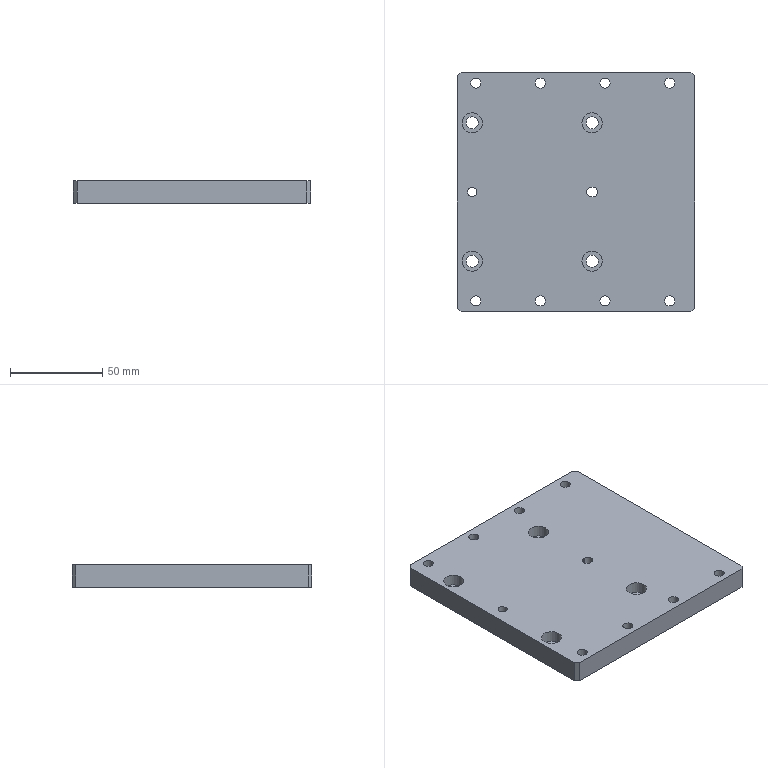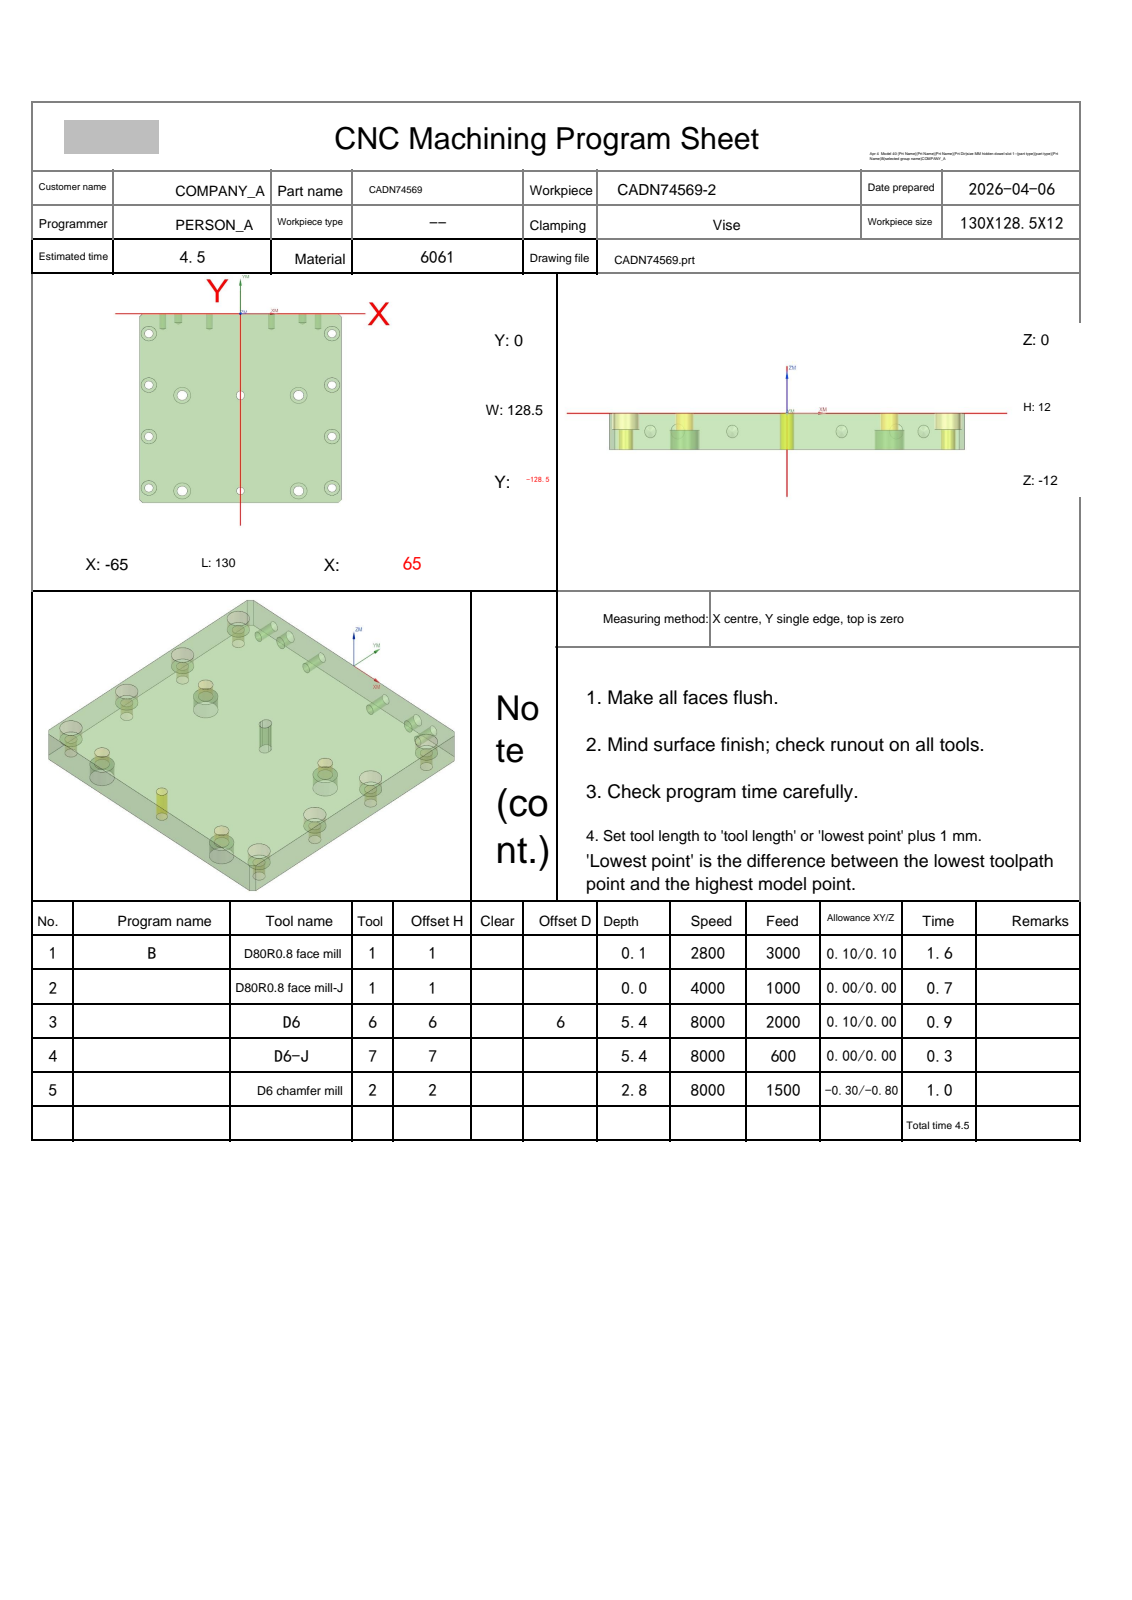NC program | NX | posted by the shop | part box 128.5 x 130 x 12 mm
Whole program:
%
O0001
(Machine time: 5.45 MIN)
(===Total Tool:4===)
(T1=D80R0.8 face mill D=80.  R=0.8  D-  H01 Z=-0.   )
(T6=D6      D=6.   R=0.   D6  H06 Z=-5.4  )
(T7=D6-J    D=6.   R=0.   D-  H07 Z=-5.4  )
(T2=D6 chamfer mill   D=6.   R=0.   D-  H02 Z=-2.8  )
G80 G90 G17 G49 G40
G91 G28 Z0
M01
N1 T01 M06
(D80R0.8 face mill  D=80. R=0.8 H=01 ce=0.10 di=0.10)
G00 G90 G54 X-117.097 Y-23.903 M03 S2800
G43 H01 Z20.
M08
Z4.517
G01 Z2.517 F3000.
X-105.097
X97.897
G02 X105.097 Y-31.103 I0.0 J-7.2
G01 Y-52.57
G02 X97.097 Y-60.57 I-8. J0.0
G01 X-97.897
G03 X-105.097 Y-67.77 I0.0 J-7.2
G01 Y-89.237
G03 X-97.097 Y-97.237 I8. J0.0
G01 X105.097
X117.097
Z4.517
G00 X-117.097 Y-23.903
Z4.033
G01 Z2.033
X-105.097
X97.897
G02 X105.097 Y-31.103 I0.0 J-7.2
G01 Y-52.57
G02 X97.097 Y-60.57 I-8. J0.0
G01 X-97.897
G03 X-105.097 Y-67.77 I0.0 J-7.2
G01 Y-89.237
G03 X-97.097 Y-97.237 I8. J0.0
G01 X105.097
X117.097
Z4.033
G00 X-117.097 Y-23.903
Z3.55
G01 Z1.55
X-105.097
X97.897
G02 X105.097 Y-31.103 I0.0 J-7.2
G01 Y-52.57
G02 X97.097 Y-60.57 I-8. J0.0
G01 X-97.897
G03 X-105.097 Y-67.77 I0.0 J-7.2
G01 Y-89.237
G03 X-97.097 Y-97.237 I8. J0.0
G01 X105.097
X117.097
Z3.55
G00 X-117.097 Y-23.903
Z3.067
G01 Z1.067
X-105.097
X97.897
G02 X105.097 Y-31.103 I0.0 J-7.2
G01 Y-52.57
G02 X97.097 Y-60.57 I-8. J0.0
G01 X-97.897
G03 X-105.097 Y-67.77 I0.0 J-7.2
G01 Y-89.237
G03 X-97.097 Y-97.237 I8. J0.0
G01 X105.097
X117.097
Z3.067
G00 Z20.
X-117.097 Y-23.903
Z2.583
G01 Z.583
X-105.097
X97.897
G02 X105.097 Y-31.103 I0.0 J-7.2
G01 Y-52.57
G02 X97.097 Y-60.57 I-8. J0.0
G01 X-97.897
G03 X-105.097 Y-67.77 I0.0 J-7.2
G01 Y-89.237
G03 X-97.097 Y-97.237 I8. J0.0
G01 X105.097
X117.097
Z2.583
G00 Z20.
X-117.097 Y-23.903
Z2.1
G01 Z.1
X-105.097
X97.897
G02 X105.097 Y-31.103 I0.0 J-7.2
G01 Y-52.57
G02 X97.097 Y-60.57 I-8. J0.0
G01 X-97.897
G03 X-105.097 Y-67.77 I0.0 J-7.2
G01 Y-89.237
G03 X-97.097 Y-97.237 I8. J0.0
G01 X105.097
X117.097
Z2.1
G00 Z20.
G91 G28 Z0.0
M05
M09
G91 G28 Z0.0
M01
N2 T01 M06
(D80R0.8 face mill-J  D=80. R=0.8 H=01 ce=0.00 di=0.00)
G00 G90 G54 X-116.999 Y-24.001 M03 S4000
G43 H01 Z20.
M08
Z2.
G01 Z0.0 F1000.
X-104.999
X97.799
G02 X104.999 Y-31.201 I0.0 J-7.2
G01 Y-52.57
G02 X96.999 Y-60.57 I-8. J0.0
G01 X-97.799
G03 X-104.999 Y-67.77 I0.0 J-7.2
G01 Y-89.139
G03 X-96.999 Y-97.139 I8. J0.0
G01 X104.999
X116.999
Z2.
G00 Z20.
G91 G28 Z0.0
M05
M09
G91 G28 Z0.0
M01
N3 T06 M06
(D6  D=6. R=0. H=06 ce=0.10 di=0.00)
G00 G90 G54 X59. Y-118.5 M03 S8000
G43 H06 Z20.
M08
Z.3
G41 D06
G01 X59.1 Y-118.507 F2000.
G03 X59.956 Y-117.556 I-.1 J.951
X59. Y-116.6 I-.956 J0.0
X59. Y-116.6 Z-.05 I0.0 J-1.9
X59. Y-116.6 Z-.4 I0.0 J-1.9
X59. Y-116.6 Z-.75 I0.0 J-1.9
X59. Y-116.6 Z-1.1 I0.0 J-1.9
X59. Y-116.6 Z-1.45 I0.0 J-1.9
X59. Y-116.6 Z-1.8 I0.0 J-1.9
X59. Y-116.6 Z-2.15 I0.0 J-1.9
X59. Y-116.6 Z-2.5 I0.0 J-1.9
X59. Y-116.6 Z-2.85 I0.0 J-1.9
X59. Y-116.6 Z-3.2 I0.0 J-1.9
X59. Y-116.6 Z-3.55 I0.0 J-1.9
X59. Y-116.6 Z-3.9 I0.0 J-1.9
X59. Y-116.6 Z-4.25 I0.0 J-1.9
X59. Y-116.6 Z-4.6 I0.0 J-1.9
X59. Y-116.6 Z-4.95 I0.0 J-1.9
X59. Y-116.6 Z-5.3 I0.0 J-1.9
X57.148 Y-118.923 Z-5.4 I0.0 J-1.9
X59. Y-120.4 I1.852 J.423
X60.9 Y-118.5 I0.0 J1.9
X59. Y-116.6 I-1.9 J0.0
X57.1 Y-118.5 I0.0 J-1.9
X57.148 Y-118.923 I1.9 J0.0
X58.08 Y-119.666 I.932 J.213
X59.036 Y-118.71 I0.0 J.956
G01 X59.029 Y-118.596
G40 X59. Y-118.5
G00 Z20.
Y-83.5
Z.3
G41 D06
G01 X59.1 Y-83.507
G03 X59.956 Y-82.556 I-.1 J.951
X59. Y-81.6 I-.956 J0.0
X59. Y-81.6 Z-.05 I0.0 J-1.9
X59. Y-81.6 Z-.4 I0.0 J-1.9
X59. Y-81.6 Z-.75 I0.0 J-1.9
X59. Y-81.6 Z-1.1 I0.0 J-1.9
X59. Y-81.6 Z-1.45 I0.0 J-1.9
X59. Y-81.6 Z-1.8 I0.0 J-1.9
X59. Y-81.6 Z-2.15 I0.0 J-1.9
X59. Y-81.6 Z-2.5 I0.0 J-1.9
X59. Y-81.6 Z-2.85 I0.0 J-1.9
X59. Y-81.6 Z-3.2 I0.0 J-1.9
X59. Y-81.6 Z-3.55 I0.0 J-1.9
X59. Y-81.6 Z-3.9 I0.0 J-1.9
X59. Y-81.6 Z-4.25 I0.0 J-1.9
X59. Y-81.6 Z-4.6 I0.0 J-1.9
X59. Y-81.6 Z-4.95 I0.0 J-1.9
X59. Y-81.6 Z-5.3 I0.0 J-1.9
X57.148 Y-83.923 Z-5.4 I0.0 J-1.9
X59. Y-85.4 I1.852 J.423
X60.9 Y-83.5 I0.0 J1.9
X59. Y-81.6 I-1.9 J0.0
X57.1 Y-83.5 I0.0 J-1.9
X57.148 Y-83.923 I1.9 J0.0
X58.08 Y-84.666 I.932 J.213
X59.036 Y-83.71 I0.0 J.956
G01 X59.029 Y-83.596
G40 X59. Y-83.5
G00 Z20.
Y-48.5
Z.3
G41 D06
G01 X59.1 Y-48.507
G03 X59.956 Y-47.556 I-.1 J.951
X59. Y-46.6 I-.956 J0.0
X59. Y-46.6 Z-.05 I0.0 J-1.9
X59. Y-46.6 Z-.4 I0.0 J-1.9
X59. Y-46.6 Z-.75 I0.0 J-1.9
X59. Y-46.6 Z-1.1 I0.0 J-1.9
X59. Y-46.6 Z-1.45 I0.0 J-1.9
X59. Y-46.6 Z-1.8 I0.0 J-1.9
X59. Y-46.6 Z-2.15 I0.0 J-1.9
X59. Y-46.6 Z-2.5 I0.0 J-1.9
X59. Y-46.6 Z-2.85 I0.0 J-1.9
X59. Y-46.6 Z-3.2 I0.0 J-1.9
X59. Y-46.6 Z-3.55 I0.0 J-1.9
X59. Y-46.6 Z-3.9 I0.0 J-1.9
X59. Y-46.6 Z-4.25 I0.0 J-1.9
X59. Y-46.6 Z-4.6 I0.0 J-1.9
X59. Y-46.6 Z-4.95 I0.0 J-1.9
X59. Y-46.6 Z-5.3 I0.0 J-1.9
X57.148 Y-48.923 Z-5.4 I0.0 J-1.9
X59. Y-50.4 I1.852 J.423
X60.9 Y-48.5 I0.0 J1.9
X59. Y-46.6 I-1.9 J0.0
X57.1 Y-48.5 I0.0 J-1.9
X57.148 Y-48.923 I1.9 J0.0
X58.08 Y-49.666 I.932 J.213
X59.036 Y-48.71 I0.0 J.956
G01 X59.029 Y-48.596
G40 X59. Y-48.5
G00 Z20.
Y-13.5
Z.3
G41 D06
G01 X59.1 Y-13.507
G03 X59.956 Y-12.556 I-.1 J.951
X59. Y-11.6 I-.956 J0.0
X59. Y-11.6 Z-.05 I0.0 J-1.9
X59. Y-11.6 Z-.4 I0.0 J-1.9
X59. Y-11.6 Z-.75 I0.0 J-1.9
X59. Y-11.6 Z-1.1 I0.0 J-1.9
X59. Y-11.6 Z-1.45 I0.0 J-1.9
X59. Y-11.6 Z-1.8 I0.0 J-1.9
X59. Y-11.6 Z-2.15 I0.0 J-1.9
X59. Y-11.6 Z-2.5 I0.0 J-1.9
X59. Y-11.6 Z-2.85 I0.0 J-1.9
X59. Y-11.6 Z-3.2 I0.0 J-1.9
X59. Y-11.6 Z-3.55 I0.0 J-1.9
X59. Y-11.6 Z-3.9 I0.0 J-1.9
X59. Y-11.6 Z-4.25 I0.0 J-1.9
X59. Y-11.6 Z-4.6 I0.0 J-1.9
X59. Y-11.6 Z-4.95 I0.0 J-1.9
X59. Y-11.6 Z-5.3 I0.0 J-1.9
X57.148 Y-13.923 Z-5.4 I0.0 J-1.9
X59. Y-15.4 I1.852 J.423
X60.9 Y-13.5 I0.0 J1.9
X59. Y-11.6 I-1.9 J0.0
X57.1 Y-13.5 I0.0 J-1.9
X57.148 Y-13.923 I1.9 J0.0
X58.08 Y-14.666 I.932 J.213
X59.036 Y-13.71 I0.0 J.956
G01 X59.029 Y-13.596
G40 X59. Y-13.5
G00 Z20.
X-59.
Z.3
G41 D06
G01 X-58.9 Y-13.507
G03 X-58.044 Y-12.556 I-.1 J.951
X-59. Y-11.6 I-.956 J0.0
X-59. Y-11.6 Z-.05 I0.0 J-1.9
X-59. Y-11.6 Z-.4 I0.0 J-1.9
X-59. Y-11.6 Z-.75 I0.0 J-1.9
X-59. Y-11.6 Z-1.1 I0.0 J-1.9
X-59. Y-11.6 Z-1.45 I0.0 J-1.9
X-59. Y-11.6 Z-1.8 I0.0 J-1.9
X-59. Y-11.6 Z-2.15 I0.0 J-1.9
X-59. Y-11.6 Z-2.5 I0.0 J-1.9
X-59. Y-11.6 Z-2.85 I0.0 J-1.9
X-59. Y-11.6 Z-3.2 I0.0 J-1.9
X-59. Y-11.6 Z-3.55 I0.0 J-1.9
X-59. Y-11.6 Z-3.9 I0.0 J-1.9
X-59. Y-11.6 Z-4.25 I0.0 J-1.9
X-59. Y-11.6 Z-4.6 I0.0 J-1.9
X-59. Y-11.6 Z-4.95 I0.0 J-1.9
X-59. Y-11.6 Z-5.3 I0.0 J-1.9
X-60.852 Y-13.923 Z-5.4 I0.0 J-1.9
X-59. Y-15.4 I1.852 J.423
X-57.1 Y-13.5 I0.0 J1.9
X-59. Y-11.6 I-1.9 J0.0
X-60.9 Y-13.5 I0.0 J-1.9
X-60.852 Y-13.923 I1.9 J0.0
X-59.92 Y-14.666 I.932 J.213
X-58.964 Y-13.71 I0.0 J.956
G01 X-58.971 Y-13.596
G40 X-59. Y-13.5
G00 Z20.
Y-48.5
Z.3
G41 D06
G01 X-58.9 Y-48.507
G03 X-58.044 Y-47.556 I-.1 J.951
X-59. Y-46.6 I-.956 J0.0
X-59. Y-46.6 Z-.05 I0.0 J-1.9
X-59. Y-46.6 Z-.4 I0.0 J-1.9
X-59. Y-46.6 Z-.75 I0.0 J-1.9
X-59. Y-46.6 Z-1.1 I0.0 J-1.9
X-59. Y-46.6 Z-1.45 I0.0 J-1.9
X-59. Y-46.6 Z-1.8 I0.0 J-1.9
X-59. Y-46.6 Z-2.15 I0.0 J-1.9
X-59. Y-46.6 Z-2.5 I0.0 J-1.9
X-59. Y-46.6 Z-2.85 I0.0 J-1.9
X-59. Y-46.6 Z-3.2 I0.0 J-1.9
X-59. Y-46.6 Z-3.55 I0.0 J-1.9
X-59. Y-46.6 Z-3.9 I0.0 J-1.9
X-59. Y-46.6 Z-4.25 I0.0 J-1.9
X-59. Y-46.6 Z-4.6 I0.0 J-1.9
X-59. Y-46.6 Z-4.95 I0.0 J-1.9
X-59. Y-46.6 Z-5.3 I0.0 J-1.9
X-60.852 Y-48.923 Z-5.4 I0.0 J-1.9
X-59. Y-50.4 I1.852 J.423
X-57.1 Y-48.5 I0.0 J1.9
X-59. Y-46.6 I-1.9 J0.0
X-60.9 Y-48.5 I0.0 J-1.9
X-60.852 Y-48.923 I1.9 J0.0
X-59.92 Y-49.666 I.932 J.213
X-58.964 Y-48.71 I0.0 J.956
G01 X-58.971 Y-48.596
G40 X-59. Y-48.5
G00 Z20.
Y-83.5
Z.3
G41 D06
G01 X-58.9 Y-83.507
G03 X-58.044 Y-82.556 I-.1 J.951
X-59. Y-81.6 I-.956 J0.0
X-59. Y-81.6 Z-.05 I0.0 J-1.9
X-59. Y-81.6 Z-.4 I0.0 J-1.9
X-59. Y-81.6 Z-.75 I0.0 J-1.9
X-59. Y-81.6 Z-1.1 I0.0 J-1.9
X-59. Y-81.6 Z-1.45 I0.0 J-1.9
X-59. Y-81.6 Z-1.8 I0.0 J-1.9
X-59. Y-81.6 Z-2.15 I0.0 J-1.9
X-59. Y-81.6 Z-2.5 I0.0 J-1.9
X-59. Y-81.6 Z-2.85 I0.0 J-1.9
X-59. Y-81.6 Z-3.2 I0.0 J-1.9
X-59. Y-81.6 Z-3.55 I0.0 J-1.9
X-59. Y-81.6 Z-3.9 I0.0 J-1.9
X-59. Y-81.6 Z-4.25 I0.0 J-1.9
X-59. Y-81.6 Z-4.6 I0.0 J-1.9
X-59. Y-81.6 Z-4.95 I0.0 J-1.9
X-59. Y-81.6 Z-5.3 I0.0 J-1.9
X-60.852 Y-83.923 Z-5.4 I0.0 J-1.9
X-59. Y-85.4 I1.852 J.423
X-57.1 Y-83.5 I0.0 J1.9
X-59. Y-81.6 I-1.9 J0.0
X-60.9 Y-83.5 I0.0 J-1.9
X-60.852 Y-83.923 I1.9 J0.0
X-59.92 Y-84.666 I.932 J.213
X-58.964 Y-83.71 I0.0 J.956
G01 X-58.971 Y-83.596
G40 X-59. Y-83.5
G00 Z20.
Y-118.5
Z.3
G41 D06
G01 X-58.9 Y-118.507
G03 X-58.044 Y-117.556 I-.1 J.951
X-59. Y-116.6 I-.956 J0.0
X-59. Y-116.6 Z-.05 I0.0 J-1.9
X-59. Y-116.6 Z-.4 I0.0 J-1.9
X-59. Y-116.6 Z-.75 I0.0 J-1.9
X-59. Y-116.6 Z-1.1 I0.0 J-1.9
X-59. Y-116.6 Z-1.45 I0.0 J-1.9
X-59. Y-116.6 Z-1.8 I0.0 J-1.9
X-59. Y-116.6 Z-2.15 I0.0 J-1.9
X-59. Y-116.6 Z-2.5 I0.0 J-1.9
X-59. Y-116.6 Z-2.85 I0.0 J-1.9
X-59. Y-116.6 Z-3.2 I0.0 J-1.9
X-59. Y-116.6 Z-3.55 I0.0 J-1.9
X-59. Y-116.6 Z-3.9 I0.0 J-1.9
X-59. Y-116.6 Z-4.25 I0.0 J-1.9
X-59. Y-116.6 Z-4.6 I0.0 J-1.9
X-59. Y-116.6 Z-4.95 I0.0 J-1.9
X-59. Y-116.6 Z-5.3 I0.0 J-1.9
X-60.852 Y-118.923 Z-5.4 I0.0 J-1.9
X-59. Y-120.4 I1.852 J.423
X-57.1 Y-118.5 I0.0 J1.9
X-59. Y-116.6 I-1.9 J0.0
X-60.9 Y-118.5 I0.0 J-1.9
X-60.852 Y-118.923 I1.9 J0.0
X-59.92 Y-119.666 I.932 J.213
X-58.964 Y-118.71 I0.0 J.956
G01 X-58.971 Y-118.596
G40 X-59. Y-118.5
G00 Z20.
G91 G28 Z0.0
M05
M09
G91 G28 Z0.0
M01
N4 T07 M06
(D6-J  D=6. R=0. H=07 ce=0.00 di=0.00)
G00 G90 G54 X59. Y-118.5 M03 S8000
G43 H07 Z20.
M08
Z-5.4
G01 X59.351 Y-116.939 F600.
X59.36 Y-116.86
G03 X59. Y-116.5 I-.36 J0.0
X57. Y-118.5 I0.0 J-2.
X59. Y-120.5 I2. J0.0
X61. Y-118.5 I0.0 J2.
X59. Y-116.5 I-2. J0.0
X58.505 Y-116.562 I0.0 J-2.
X58.234 Y-116.911 I.089 J-.349
G01 X58.274 Y-117.074
X59. Y-118.5
G00 Z20.
Y-83.5
Z-5.4
G01 X59.351 Y-81.939
X59.36 Y-81.86
G03 X59. Y-81.5 I-.36 J0.0
X57. Y-83.5 I0.0 J-2.
X59. Y-85.5 I2. J0.0
X61. Y-83.5 I0.0 J2.
X59. Y-81.5 I-2. J0.0
X58.505 Y-81.562 I0.0 J-2.
X58.234 Y-81.911 I.089 J-.349
G01 X58.274 Y-82.074
X59. Y-83.5
G00 Z20.
Y-48.5
Z-5.4
G01 X59.351 Y-46.939
X59.36 Y-46.86
G03 X59. Y-46.5 I-.36 J0.0
X57. Y-48.5 I0.0 J-2.
X59. Y-50.5 I2. J0.0
X61. Y-48.5 I0.0 J2.
X59. Y-46.5 I-2. J0.0
X58.505 Y-46.562 I0.0 J-2.
X58.234 Y-46.911 I.089 J-.349
G01 X58.274 Y-47.074
X59. Y-48.5
G00 Z20.
Y-13.5
Z-5.4
G01 X59.351 Y-11.939
X59.36 Y-11.86
G03 X59. Y-11.5 I-.36 J0.0
X57. Y-13.5 I0.0 J-2.
X59. Y-15.5 I2. J0.0
X61. Y-13.5 I0.0 J2.
X59. Y-11.5 I-2. J0.0
X58.505 Y-11.562 I0.0 J-2.
X58.234 Y-11.911 I.089 J-.349
G01 X58.274 Y-12.074
X59. Y-13.5
G00 Z20.
X-59.
Z-5.4
G01 X-58.649 Y-11.939
X-58.64 Y-11.86
G03 X-59. Y-11.5 I-.36 J0.0
X-61. Y-13.5 I0.0 J-2.
X-59. Y-15.5 I2. J0.0
X-57. Y-13.5 I0.0 J2.
X-59. Y-11.5 I-2. J0.0
X-59.495 Y-11.562 I0.0 J-2.
X-59.766 Y-11.911 I.089 J-.349
G01 X-59.726 Y-12.074
X-59. Y-13.5
G00 Z20.
Y-48.5
Z-5.4
G01 X-58.649 Y-46.939
X-58.64 Y-46.86
G03 X-59. Y-46.5 I-.36 J0.0
X-61. Y-48.5 I0.0 J-2.
X-59. Y-50.5 I2. J0.0
X-57. Y-48.5 I0.0 J2.
X-59. Y-46.5 I-2. J0.0
X-59.495 Y-46.562 I0.0 J-2.
X-59.766 Y-46.911 I.089 J-.349
G01 X-59.726 Y-47.074
X-59. Y-48.5
G00 Z20.
Y-83.5
Z-5.4
G01 X-58.649 Y-81.939
X-58.64 Y-81.86
G03 X-59. Y-81.5 I-.36 J0.0
X-61. Y-83.5 I0.0 J-2.
X-59. Y-85.5 I2. J0.0
X-57. Y-83.5 I0.0 J2.
X-59. Y-81.5 I-2. J0.0
X-59.495 Y-81.562 I0.0 J-2.
X-59.766 Y-81.911 I.089 J-.349
G01 X-59.726 Y-82.074
X-59. Y-83.5
G00 Z20.
Y-118.5
Z-5.4
G01 X-58.649 Y-116.939
X-58.64 Y-116.86
G03 X-59. Y-116.5 I-.36 J0.0
X-61. Y-118.5 I0.0 J-2.
X-59. Y-120.5 I2. J0.0
X-57. Y-118.5 I0.0 J2.
X-59. Y-116.5 I-2. J0.0
X-59.495 Y-116.562 I0.0 J-2.
X-59.766 Y-116.911 I.089 J-.349
G01 X-59.726 Y-117.074
X-59. Y-118.5
G00 Z20.
G91 G28 Z0.0
M05
M09
G91 G28 Z0.0
M01
N5 T02 M06
(D6 chamfer mill  D=6. R=0. H=02 ce=0.00 di=0.00)
G00 G90 G54 X0.0 Y-120.5 M03 S8000
G43 H02 Z20.
M08
G98 G81 X0.0 Y-120.5 Z-2.8 R3. F1000.
G80
G00 Z20.
G00 G90 X36.413 Y-56.007 M03 S8000
Z20.
Z-.9
G01 Z-1.4 F1200.
X36. Y-56.2
G03 X37.5 Y-57.7 I1.5 J0.0
X39.7 Y-55.5 I0.0 J2.2
X37.5 Y-53.3 I-2.2 J0.0
X35.3 Y-55.5 I0.0 J-2.2
X37.5 Y-57.7 I2.2 J0.0
X39. Y-56.2 I0.0 J1.5
G01 X38.587 Y-56.007
Z-.9
G00 Z20.
X36.413 Y-121.007
Z-.9
G01 Z-1.4
X36. Y-121.2
G03 X37.5 Y-122.7 I1.5 J0.0
X39.7 Y-120.5 I0.0 J2.2
X37.5 Y-118.3 I-2.2 J0.0
X35.3 Y-120.5 I0.0 J-2.2
X37.5 Y-122.7 I2.2 J0.0
X39. Y-121.2 I0.0 J1.5
G01 X38.587 Y-121.007
Z-.9
G00 Z20.
X-38.587
Z-.9
G01 Z-1.4
X-39. Y-121.2
G03 X-37.5 Y-122.7 I1.5 J0.0
X-35.3 Y-120.5 I0.0 J2.2
X-37.5 Y-118.3 I-2.2 J0.0
X-39.7 Y-120.5 I0.0 J-2.2
X-37.5 Y-122.7 I2.2 J0.0
X-36. Y-121.2 I0.0 J1.5
G01 X-36.413 Y-121.007
Z-.9
G00 Z20.
X-38.587 Y-56.007
Z-.9
G01 Z-1.4
X-39. Y-56.2
G03 X-37.5 Y-57.7 I1.5 J0.0
X-35.3 Y-55.5 I0.0 J2.2
X-37.5 Y-53.3 I-2.2 J0.0
X-39.7 Y-55.5 I0.0 J-2.2
X-37.5 Y-57.7 I2.2 J0.0
X-36. Y-56.2 I0.0 J1.5
G01 X-36.413 Y-56.007
Z-.9
G00 Z20.
G00 G90 X-56.711 Y-13.271 M03 S8000
Z20.
Z-1.5
G01 Z-2. F600.
X-56. Y-13.2
G03 X-59. Y-10.2 I-3. J0.0
X-62.3 Y-13.5 I0.0 J-3.3
X-59. Y-16.8 I3.3 J0.0
X-55.7 Y-13.5 I0.0 J3.3
X-59. Y-10.2 I-3.3 J0.0
X-62. Y-13.2 I0.0 J-3.
G01 X-61.289 Y-13.271
Z-1.5
G00 Z20.
X-56.711 Y-48.271
Z-1.5
G01 Z-2.
X-56. Y-48.2
G03 X-59. Y-45.2 I-3. J0.0
X-62.3 Y-48.5 I0.0 J-3.3
X-59. Y-51.8 I3.3 J0.0
X-55.7 Y-48.5 I0.0 J3.3
X-59. Y-45.2 I-3.3 J0.0
X-62. Y-48.2 I0.0 J-3.
G01 X-61.289 Y-48.271
Z-1.5
G00 Z20.
X-56.711 Y-83.271
Z-1.5
G01 Z-2.
X-56. Y-83.2
G03 X-59. Y-80.2 I-3. J0.0
X-62.3 Y-83.5 I0.0 J-3.3
X-59. Y-86.8 I3.3 J0.0
X-55.7 Y-83.5 I0.0 J3.3
X-59. Y-80.2 I-3.3 J0.0
X-62. Y-83.2 I0.0 J-3.
G01 X-61.289 Y-83.271
Z-1.5
G00 Z20.
X-56.711 Y-118.271
Z-1.5
G01 Z-2.
X-56. Y-118.2
G03 X-59. Y-115.2 I-3. J0.0
X-62.3 Y-118.5 I0.0 J-3.3
X-59. Y-121.8 I3.3 J0.0
X-55.7 Y-118.5 I0.0 J3.3
X-59. Y-115.2 I-3.3 J0.0
X-62. Y-118.2 I0.0 J-3.
G01 X-61.289 Y-118.271
Z-1.5
G00 Z20.
X61.289
Z-1.5
G01 Z-2.
X62. Y-118.2
G03 X59. Y-115.2 I-3. J0.0
X55.7 Y-118.5 I0.0 J-3.3
X59. Y-121.8 I3.3 J0.0
X62.3 Y-118.5 I0.0 J3.3
X59. Y-115.2 I-3.3 J0.0
X56. Y-118.2 I0.0 J-3.
G01 X56.711 Y-118.271
Z-1.5
G00 Z20.
X61.289 Y-83.271
Z-1.5
G01 Z-2.
X62. Y-83.2
G03 X59. Y-80.2 I-3. J0.0
X55.7 Y-83.5 I0.0 J-3.3
X59. Y-86.8 I3.3 J0.0
X62.3 Y-83.5 I0.0 J3.3
X59. Y-80.2 I-3.3 J0.0
X56. Y-83.2 I0.0 J-3.
G01 X56.711 Y-83.271
Z-1.5
G00 Z20.
X61.289 Y-48.271
Z-1.5
G01 Z-2.
X62. Y-48.2
G03 X59. Y-45.2 I-3. J0.0
X55.7 Y-48.5 I0.0 J-3.3
X59. Y-51.8 I3.3 J0.0
X62.3 Y-48.5 I0.0 J3.3
X59. Y-45.2 I-3.3 J0.0
X56. Y-48.2 I0.0 J-3.
G01 X56.711 Y-48.271
Z-1.5
G00 Z20.
X61.289 Y-13.271
Z-1.5
G01 Z-2.
X62. Y-13.2
G03 X59. Y-10.2 I-3. J0.0
X55.7 Y-13.5 I0.0 J-3.3
X59. Y-16.8 I3.3 J0.0
X62.3 Y-13.5 I0.0 J3.3
X59. Y-10.2 I-3.3 J0.0
X56. Y-13.2 I0.0 J-3.
G01 X56.711 Y-13.271
Z-1.5
G00 Z20.
G00 G90 X-54.046 Y-129.2 M03 S7000
Z20.
Z2.5
G01 X-62.953 Z-.742 F1500.
X-63.16 Y-129.162 Z-.819
X-63.355 Y-129.081 Z-.895
X-63.528 Y-128.962 Z-.972
X-63.583 Y-128.907 Z-1.
X-65.407 Y-127.083
G02 X-65.7 Y-126.376 I.707 J.707
G01 Y-2.124
G02 X-65.407 Y-1.417 I1. J0.0
G01 X-63.583 Y.407
G02 X-62.876 Y.7 I.707 J-.707
G01 X62.876
G02 X63.583 Y.407 I0.0 J-1.
G01 X65.407 Y-1.417
G02 X65.7 Y-2.124 I-.707 J-.707
G01 Y-126.376
G02 X65.407 Y-127.083 I-1. J0.0
G01 X63.583 Y-128.907
G02 X62.876 Y-129.2 I-.707 J.707
G01 X-62.876
G02 X-63.583 Y-128.907 I0.0 J1.
G01 X-63.936 Y-128.554
Z1.5
G00 Z20.
X.836 Y-57.591
Z2.5
G01 X.931 Y-57.544 Z2.461
X1.168 Y-57.374 Z2.355
X1.374 Y-57.168 Z2.249
X1.544 Y-56.931 Z2.143
X1.674 Y-56.671 Z2.037
X1.76 Y-56.392 Z1.931
X1.8 Y-56.104 Z1.825
Y-54.896 Z1.386
X1.76 Y-54.608 Z1.28
X1.674 Y-54.329 Z1.174
X1.544 Y-54.069 Z1.068
X1.374 Y-53.832 Z.962
X1.168 Y-53.626 Z.856
X.931 Y-53.456 Z.75
X.671 Y-53.326 Z.644
X.392 Y-53.24 Z.538
X.104 Y-53.2 Z.432
X-.104 Z.356
X-.392 Y-53.24 Z.25
X-.671 Y-53.326 Z.144
X-.931 Y-53.456 Z.038
X-1.168 Y-53.626 Z-.068
X-1.374 Y-53.832 Z-.174
X-1.544 Y-54.069 Z-.28
X-1.674 Y-54.329 Z-.386
X-1.76 Y-54.608 Z-.492
X-1.8 Y-54.896 Z-.598
Y-56. Z-1.
G03 X0.0 Y-57.8 I1.8 J0.0
X1.8 Y-56. I0.0 J1.8
G01 Y-55.
G03 X0.0 Y-53.2 I-1.8 J0.0
X-1.8 Y-55. I0.0 J-1.8
G01 Y-56.
G03 X-1.731 Y-56.494 I1.8 J0.0
G01 Z1.5
G00 Z20.
M05
M09
G91 G28 Z0.0
G91 G28 Y0.0
M30
%